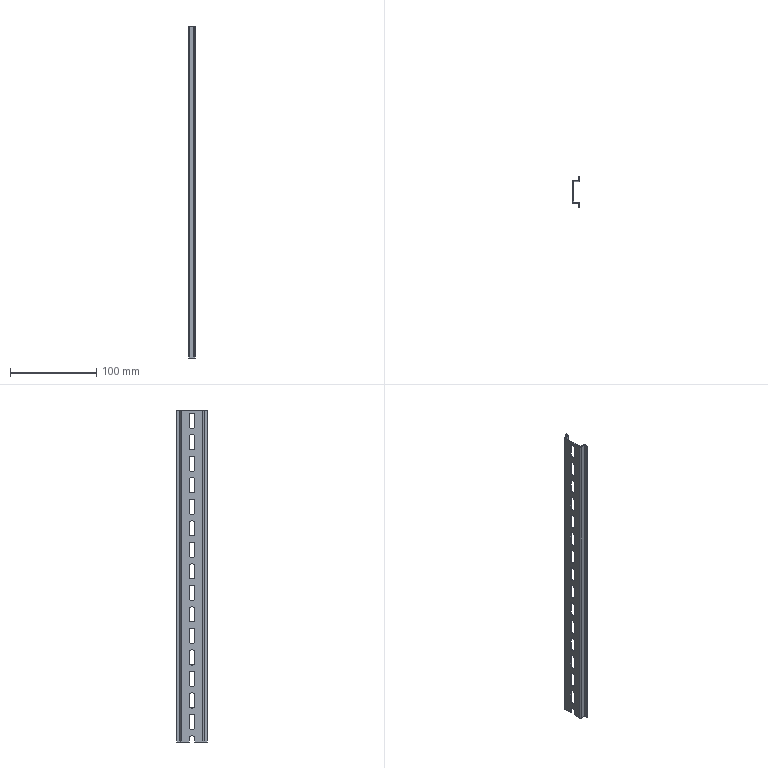Part | SolidWorks | features BaseBody 1 | 1 solid | 86 faces | box 7.5 x 35 x 386 mm | volume 16663 mm3 | plane 47 | cylinder 39 | commonest cylinder face diameters 6.3 x31 1 x4 2 x4